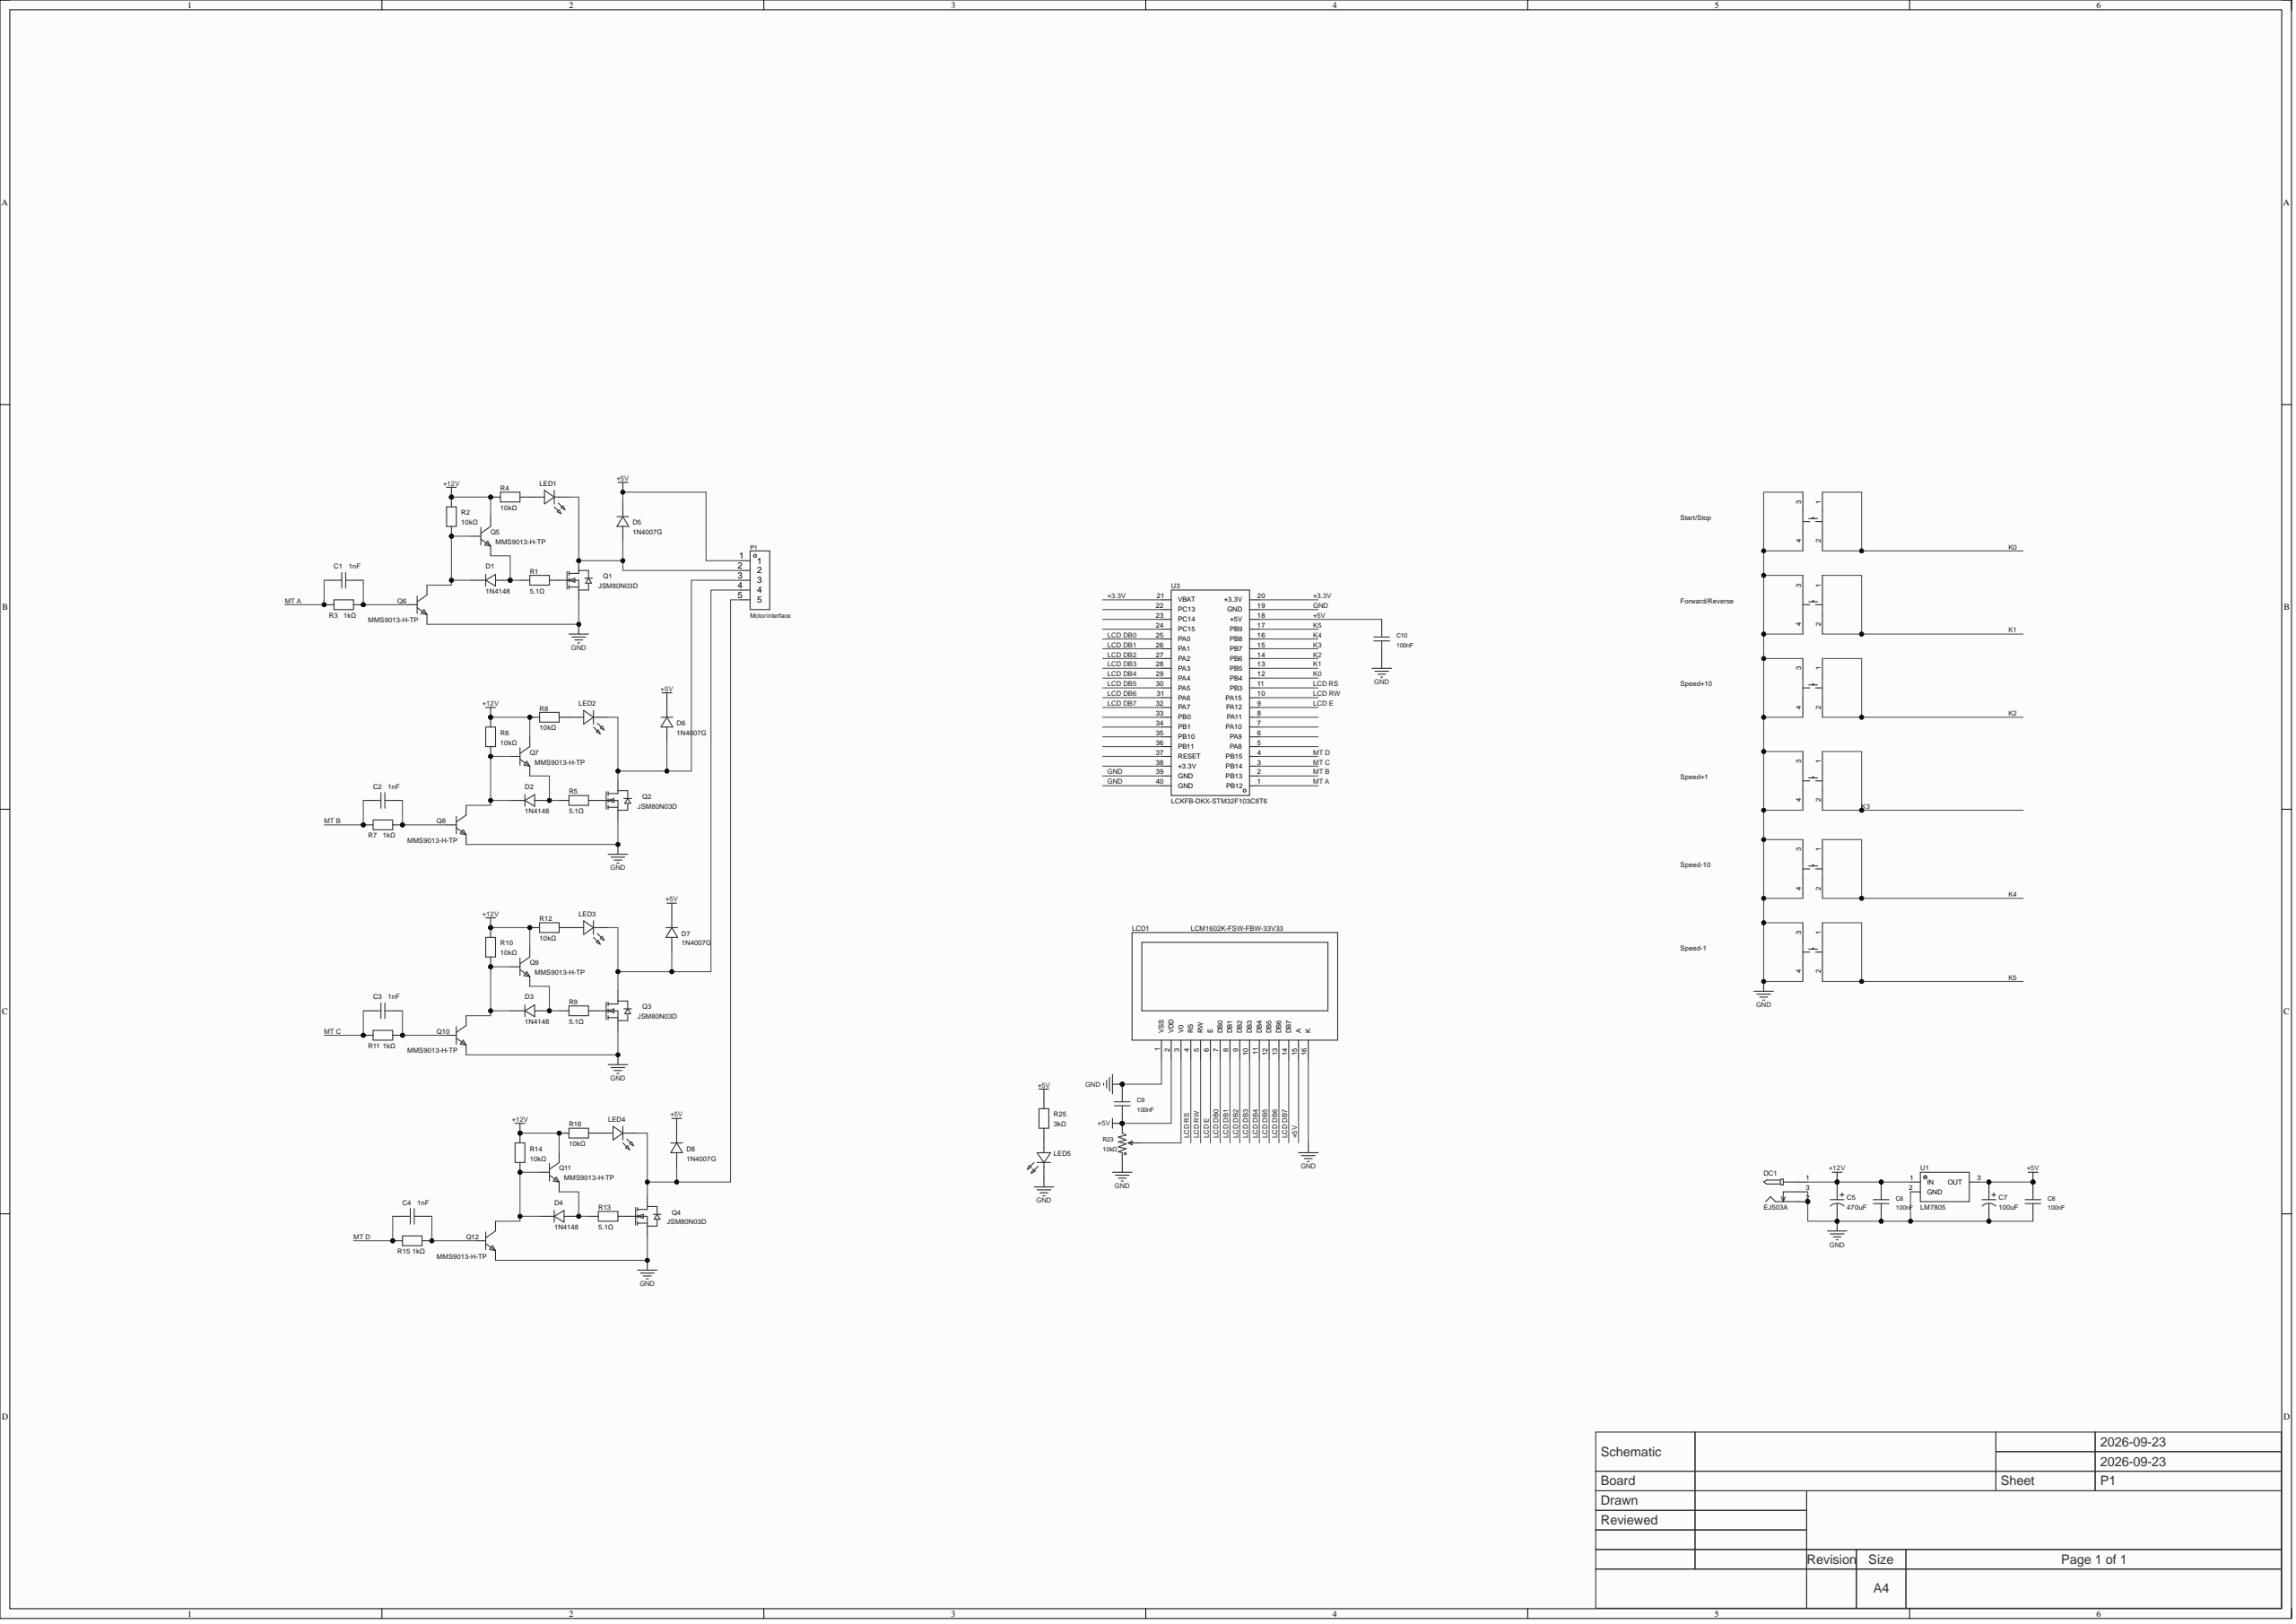Circuit board | Altium Designer | 64 parts | 51 nets
Bill of materials:
Comment,Description,Designator,Footprint,LibRef,Quantity
"1nF","Capacitance: 1nF; tolerance: ±20%; working voltage (AC): 400V; protection class: Y1;","C1, C2, C3, C4","","KY1102M400VAC70Y10093","4"
"470uF","Capacitance: 470uF; tolerance: ±20%; rated voltage: 35V; ripple current: 320mA@120Hz;","C5","","JVJ35V470M10x10","1"
"100nF","","C6, C8, C9, C10","","MPE104J100V0501","4"
"100uF","Capacitance: 100uF; tolerance: ±20%; rated voltage: 50V; ripple current: 140mA@120Hz;","C7","","JVJ50V100M6x8","1"
"1N4148","","D1, D2, D3, D4","","1N4148_C9900036548","4"
"1N4007G","Diode configuration: 1 discrete; forward voltage (Vf): 1.1V@1A; reverse voltage (Vr): 1kV; rectified current: 1A;","D5, D6, D7, D8","","1N4007G_C2457","4"
"EJ503A","","DC1","","EJ503A","1"
"Start/Stop","Circuit: SPST; button shape: round button; actuating force: 2.6N; mounting: upright SMD; switch length: 6mm; switch width: 6mm; switch height: 4.5mm; bracket: without bracket; contact current: 50mA; rated voltage: 12V; LED: -; operating life: -;","K0","","TS-1002S-04526C_1","1"
"Forward/Reverse","Circuit: SPST; button shape: round button; actuating force: 2.6N; mounting: upright SMD; switch length: 6mm; switch width: 6mm; switch height: 4.5mm; bracket: without bracket; contact current: 50mA; rated voltage: 12V; LED: -; operating life: -;","K1","","TS-1002S-04526C","1"
"Speed+10","Circuit: SPST; button shape: round button; actuating force: 2.6N; mounting: upright SMD; switch length: 6mm; switch width: 6mm; switch height: 4.5mm; bracket: without bracket; contact current: 50mA; rated voltage: 12V; LED: -; operating life: -;","K2","","TS-1002S-04526C_4","1"
"Speed+1","Circuit: SPST; button shape: round button; actuating force: 2.6N; mounting: upright SMD; switch length: 6mm; switch width: 6mm; switch height: 4.5mm; bracket: without bracket; contact current: 50mA; rated voltage: 12V; LED: -; operating life: -;","K3","","TS-1002S-04526C_2","1"
"Speed-10","Circuit: SPST; button shape: round button; actuating force: 2.6N; mounting: upright SMD; switch length: 6mm; switch width: 6mm; switch height: 4.5mm; bracket: without bracket; contact current: 50mA; rated voltage: 12V; LED: -; operating life: -;","K4","","TS-1002S-04526C_5","1"
"Speed-1","Circuit: SPST; button shape: round button; actuating force: 2.6N; mounting: upright SMD; switch length: 6mm; switch width: 6mm; switch height: 4.5mm; bracket: without bracket; contact current: 50mA; rated voltage: 12V; LED: -; operating life: -;","K5","","TS-1002S-04526C_3","1"
"LCM1602K-FSW-FBW-33V33","Controller chip: KS0066U; size (inch): -;","LCD1","","LCM1602K-FSW-FBW-33V33","1"
"3mmFIR","","LED1, LED2, LED3, LED4, LED5","","3mmFIR","5"
"Motor interface","","P1","","LAIL-PZ2.54-5P-L","1"
"JSM80N03D","Quantity: 1 N-channel; drain-source voltage (Vdss): 30V; continuous drain current (Id): 80A; on-resistance (RDS(on)): 7.5mΩ@4.5V; 4.2mΩ@10V; power dissipation (Pd): 46W; threshold voltage (Vgs(th)): 1.5V;","Q1, Q2, Q3, Q4","","JSM80N03D","4"
"MMS9013-H-TP","Transistor type: NPN; collector current (Ic): 500mA; collector-emitter breakdown voltage (Vceo): 25V; power dissipation (Pd): 300mW; DC current gain (hFE): 350;","Q5, Q6, Q7, Q8, Q9, Q10, Q11, Q12","","MMS9013-H-TP","8"
"5.1Ω","Resistor type: thick film resistor; resistance: 5.1Ω; tolerance: ±1%; power: 100mW; working voltage: 75V; temperature coefficient: ±200ppm/?;","R1, R5, R9, R13","R0603","FRC0603F5R10TS","4"
"10kΩ","Resistor type: carbon film resistor; resistance: 10kΩ; tolerance: ±5%; power: 2W; temperature coefficient: ±200ppm/?;, Resistance: 10kΩ; tolerance: ±10%; power: 500mW; temperature coefficient: ±100ppm/?;","R2, R4, R6, R8, R10, R12, R14, R16, R23","","MGR02WJ0103A10, MGR02WJ0103A10_1, 3362U-1-103LF","9"
"1kΩ","Resistor type: carbon film resistor; resistance: 1kΩ; tolerance: ±5%; power: 2W;","R3, R7, R11, R15","","MGR02WJ0102A10","4"
"3kΩ","Resistance: 3kΩ; tolerance: ±5%; power: 3W; temperature coefficient: ±50ppm/?;","R25","","TA303PA3K00JE","1"
"LM7805","Output polarity: positive; working voltage: 20V; output voltage: 5V; output current: 1A; power supply ripple rejection (PSRR): 62dB@(120Hz); output type: fixed;","U1","","LM7805_C22467097","1"
"LCKFB-DKX-STM32F103C8T6","Cortex-M3 core, 64KB program memory, 20KB total RAM, up to 72MHz clock, for efficient computing and stable operation.","U3","CONN-TH_L53.3-W22.9_STM32F103C8T6-CARD","LCKFB-DKX-STM32F103C8T6","1"
Netlist (Protel format):
[
C1

1nF



]
[
C2

1nF



]
[
C3

1nF



]
[
C4

1nF



]
[
C5

470uF



]
[
C6

100nF



]
[
C7

100uF



]
[
C8

100nF



]
[
C9

100nF



]
[
C10

100nF



]
[
D1

1N4148



]
[
D2

1N4148



]
[
D3

1N4148



]
[
D4

1N4148



]
[
D5

1N4007G



]
[
D6

1N4007G



]
[
D7

1N4007G



]
[
D8

1N4007G



]
[
DC1

EJ503A



]
[
K0

Start/Stop



]
[
K1

Forward/Reverse



]
[
K2

Speed+10



]
[
K3

Speed+1



]
[
K4

Speed-10



]
[
K5

Speed-1



]
[
LCD1

LCM1602K-FSW-FBW-33V33



]
[
LED1

3mmFIR



]
[
LED2

3mmFIR



]
[
LED3

3mmFIR



]
[
LED4

3mmFIR



]
[
LED5

3mmFIR



]
[
P1

Motor interface



]
[
Q1

JSM80N03D



]
[
Q2

JSM80N03D



]
[
Q3

JSM80N03D



]
[
Q4

JSM80N03D



]
[
Q5

MMS9013-H-TP



]
[
Q6

MMS9013-H-TP



]
[
Q7

MMS9013-H-TP



]
[
Q8

MMS9013-H-TP



]
[
Q9

MMS9013-H-TP



]
[
Q10

MMS9013-H-TP



]
[
Q11

MMS9013-H-TP



]
[
Q12

MMS9013-H-TP



]
[
R1
R0603
5.1Ω



]
[
R2

10kΩ



]
[
R3

1kΩ



]
[
R4

10kΩ



]
[
R5
R0603
5.1Ω



]
[
R6

10kΩ



]
[
R7

1kΩ



]
[
R8

10kΩ



]
[
R9
R0603
5.1Ω



]
[
R10

10kΩ



]
[
R11

1kΩ



]
[
R12

10kΩ



]
[
R13
R0603
5.1Ω



]
[
R14

10kΩ



]
[
R15

1kΩ



]
[
R16

10kΩ



]
[
R23

10kΩ



]
[
R25

3kΩ



]
[
U1

LM7805



]
[
U3
CONN-TH_L53.3-W22.9_STM32F103C8T6-CARD
LCKFB-DKX-STM32F103C8T6



]
(
NetQ4_1
Q4-1
R13-2
)
(
NetQ3_1
Q3-1
R9-2
)
(
NetQ2_1
Q2-1
R5-2
)
(
NetQ1_1
Q1-1
R1-2
)
(
NetLED5_1
LED5-1
R25-1
)
(
NetLED4_1
LED4-1
R16-2
)
(
NetLED3_1
LED3-1
R12-2
)
(
NetLED2_1
LED2-1
R8-2
)
(
NetLED1_1
LED1-1
R4-2
)
(
NetLCD1_3
LCD1-3
R23-2
)
(
NetD8_2
D8-2
LED4-2
P1-5
Q4-2
)
(
NetD7_2
D7-2
LED3-2
P1-4
Q3-2
)
(
NetD6_2
D6-2
LED2-2
P1-3
Q2-2
)
(
NetD5_2
D5-2
LED1-2
P1-2
Q1-2
)
(
NetD4_2
D4-2
Q11-1
Q12-3
R14-1
)
(
NetD4_1
D4-1
Q11-2
R13-1
)
(
NetD3_2
D3-2
Q9-1
Q10-3
R10-1
)
(
NetD3_1
D3-1
Q9-2
R9-1
)
(
NetD2_2
D2-2
Q7-1
Q8-3
R6-1
)
(
NetD2_1
D2-1
Q7-2
R5-1
)
(
NetD1_2
D1-2
Q5-1
Q6-3
R2-1
)
(
NetD1_1
D1-1
Q5-2
R1-1
)
(
NetC4_2
C4-2
Q12-1
R15-2
)
(
NetC3_2
C3-2
Q10-1
R11-2
)
(
NetC2_2
C2-2
Q8-1
R7-2
)
(
NetC1_2
C1-2
Q6-1
R3-2
)
(
MT D
C4-1
R15-1
U3-4
)
(
MT C
C3-1
R11-1
U3-3
)
(
MT B
C2-1
R7-1
U3-2
)
(
MT A
C1-1
R3-1
U3-1
)
(
LCD RW
LCD1-5
U3-10
)
(
LCD RS
LCD1-4
U3-11
)
(
LCD E
LCD1-6
U3-9
)
(
LCD DB7
LCD1-14
U3-32
)
(
LCD DB6
LCD1-13
U3-31
)
(
LCD DB5
LCD1-12
U3-30
)
(
LCD DB4
LCD1-11
U3-29
)
(
LCD DB3
LCD1-10
U3-28
)
(
LCD DB2
LCD1-9
U3-27
)
(
LCD DB1
LCD1-8
U3-26
)
(
LCD DB0
LCD1-7
U3-25
)
(
K5
K5-1
K5-2
U3-17
)
(
K4
K4-1
K4-2
U3-16
)
(
K3
K3-1
K3-2
U3-15
)
(
K2
K2-1
K2-2
U3-14
)
(
K1
K1-1
K1-2
U3-13
)
(
K0
K0-1
K0-2
U3-12
)
(
GND
C5-2
C6-1
C7-2
C8-1
C9-1
C10-2
DC1-2
DC1-3
K0-3
K0-4
K1-3
K1-4
K2-3
K2-4
K3-3
K3-4
K4-3
K4-4
K5-3
K5-4
LCD1-1
LCD1-16
LED5-2
Q1-3
Q2-3
Q3-3
Q4-3
Q6-2
Q8-2
Q10-2
Q12-2
R23-1
U1-2
U3-19
U3-39
U3-40
)
(
+12V
C5-1
C6-2
DC1-1
Q5-3
Q7-3
Q9-3
Q11-3
R2-2
R4-1
R6-2
R8-1
R10-2
R12-1
R14-2
R16-1
U1-1
)
(
+5V
C7-1
C8-2
C9-2
C10-1
D5-1
D6-1
D7-1
D8-1
LCD1-2
LCD1-15
P1-1
R23-3
R25-2
U1-3
U3-18
)
(
+3.3V
U3-20
U3-21
)